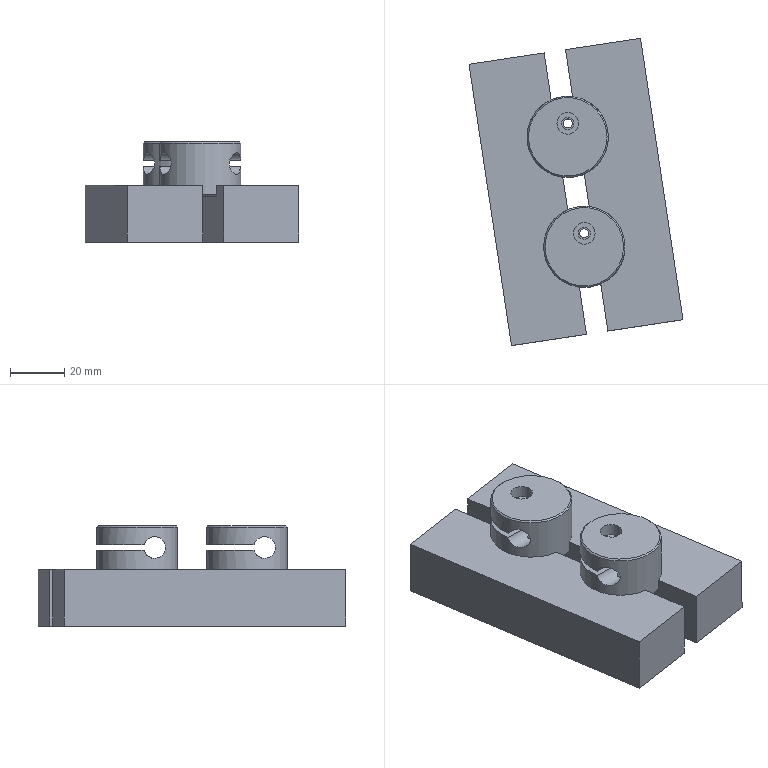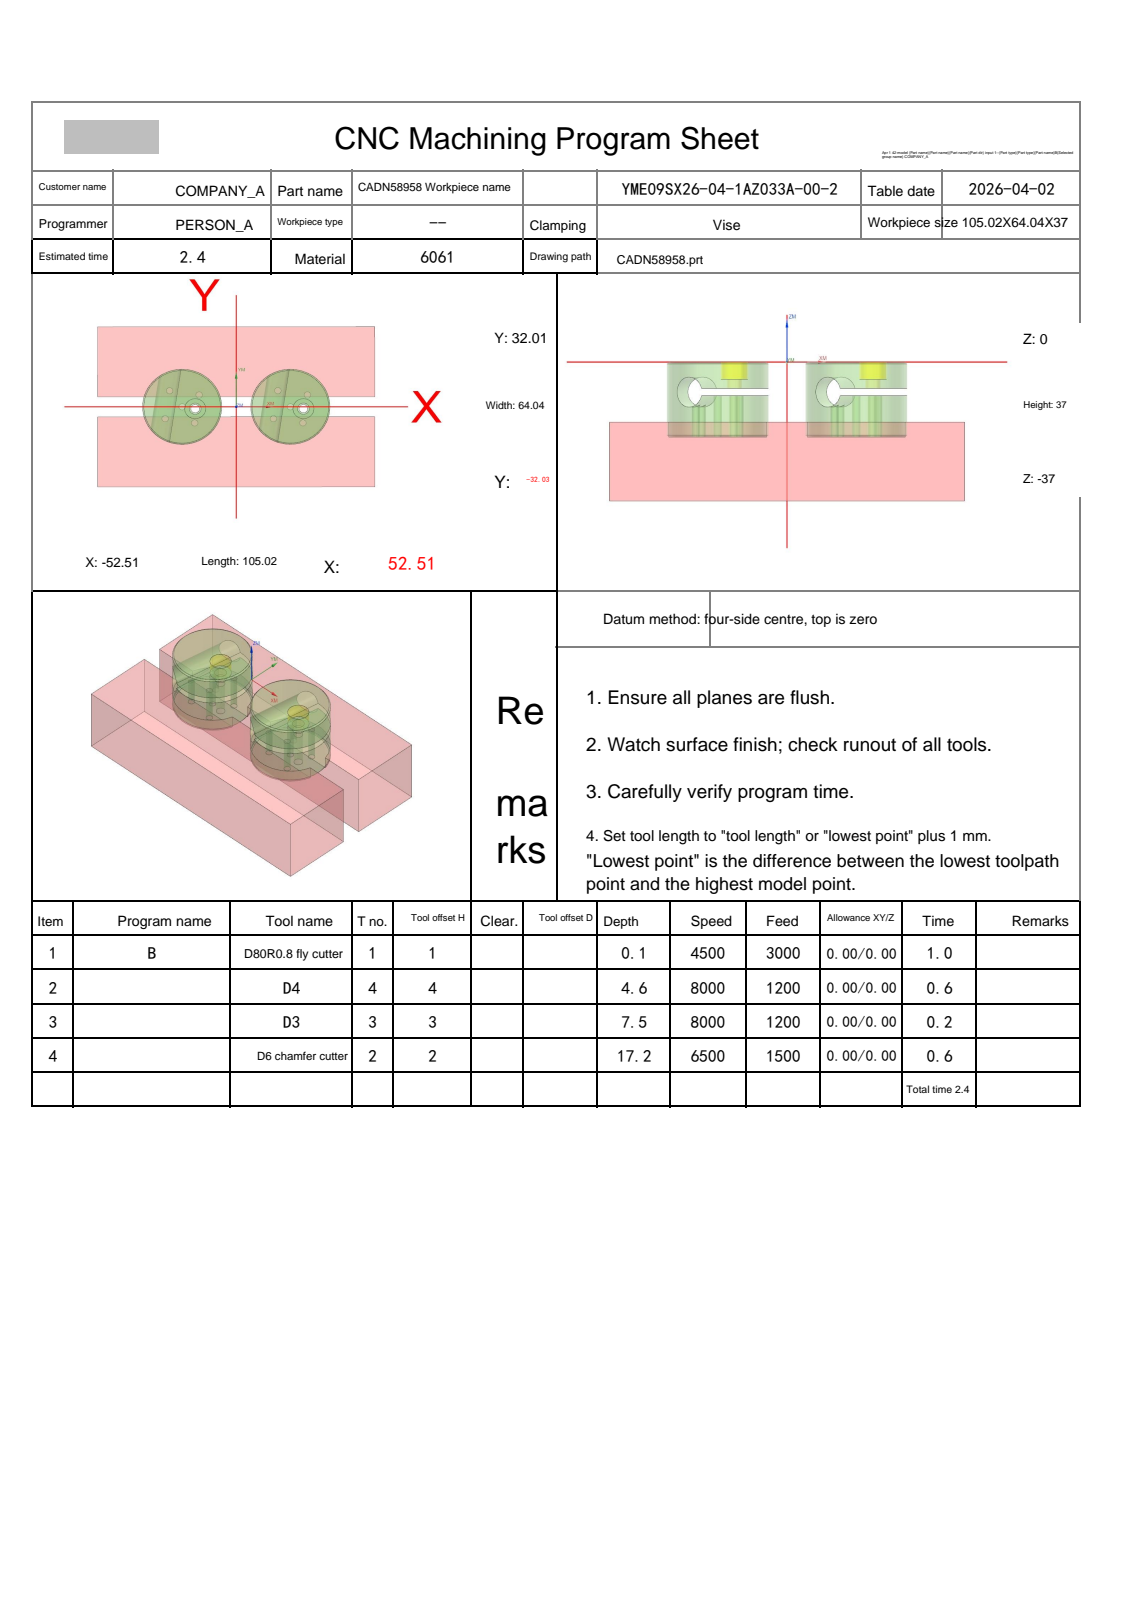NC program | NX | posted by the shop | part box 78.946 x 113.372 x 37 mm
Whole program:
%
O0001
(Machine time: 3.09 MIN)
(===Total Tool:4===)
(T1=D80R0.8 fly cutter D=80.  R=0.8  D-  H01 Z=0.    )
(T4=D4      D=4.   R=0.   D4  H04 Z=-4.6  )
(T3=D3      D=3.   R=0.   D3  H03 Z=-7.5  )
(T2=D6 chamfer cutter   D=6.   R=0.   D-  H02 Z=-17.2 )
G80 G90 G17 G49 G40
G91 G28 Z0
M01
N1 T01 M06
(D80R0.8 fly cutter  D=80. R=0.8 H=01 ce=0.20 di=0.10)
G00 G90 G54 X-104.523 Y-.009 M03 S4500
G43 H01 Z50.
M08
Z6.011
G01 Z4.011 F3000.
X-92.523
X92.529
X104.529
Z6.011
G00 Z7.5
X-104.523
Z5.522
G01 Z3.522
X-92.523
X92.529
X104.529
Z5.522
G00 Z7.011
X-104.523
Z5.033
G01 Z3.033
X-92.523
X92.529
X104.529
Z5.033
G00 Z6.522
X-104.523
Z4.544
G01 Z2.544
X-92.523
X92.529
X104.529
Z4.544
G00 Z6.033
X-104.523
Z4.056
G01 Z2.056
X-92.523
X92.529
X104.529
Z4.056
G00 Z5.544
X-104.523
Z3.567
G01 Z1.567
X-92.523
X92.529
X104.529
Z3.567
G00 Z5.056
X-104.523
Z3.078
G01 Z1.078
X-92.523
X92.529
X104.529
Z3.078
G00 Z4.567
X-104.523
Z2.589
G01 Z.589
X-92.523
X92.529
X104.529
Z2.589
G00 Z4.078
X-104.523
Z2.1
G01 Z.1
X-92.523
X92.529
X104.529
Z2.1
G00 Z50.
G00 G90 X-104.523 Y-.009 M03 S4500
Z50.
Z2.
G01 Z0.0 F1000.
X-92.523
X92.529
X104.529
Z2.
G00 Z50.
G91 G28 Z0.0
M05
M09
G91 G28 Z0.0
M01
N2 T04 M06
(D4  D=4. R=0. H=04 ce=0.05 di=0.00)
G00 G90 G54 X25.447 Y-.745 M03 S8000
G43 H04 Z50.
M08
Z.5
G01 X25.302 Y-.734 F1200.
G03 X24.327 Y-1.709 I0.0 J-.975
X25.157 Y-2.673 I.975 J0.0
X25.157 Y-2.673 Z.2 I.29 J1.928
X25.157 Y-2.673 Z-.1 I.29 J1.928
X25.157 Y-2.673 Z-.4 I.29 J1.928
X25.157 Y-2.673 Z-.7 I.29 J1.928
X25.157 Y-2.673 Z-1. I.29 J1.928
X25.157 Y-2.673 Z-1.3 I.29 J1.928
X25.157 Y-2.673 Z-1.6 I.29 J1.928
X25.157 Y-2.673 Z-1.9 I.29 J1.928
X25.157 Y-2.673 Z-2.2 I.29 J1.928
X25.157 Y-2.673 Z-2.5 I.29 J1.928
X25.157 Y-2.673 Z-2.8 I.29 J1.928
X25.157 Y-2.673 Z-3.1 I.29 J1.928
X25.157 Y-2.673 Z-3.4 I.29 J1.928
X25.157 Y-2.673 Z-3.7 I.29 J1.928
X25.157 Y-2.673 Z-4. I.29 J1.928
X25.157 Y-2.673 Z-4.3 I.29 J1.928
X25.157 Y-2.673 Z-4.6 I.29 J1.928
X25.447 Y-2.695 I.29 J1.928
X27.397 Y-.745 I0.0 J1.95
X25.447 Y1.205 I-1.95 J0.0
X23.497 Y-.745 I0.0 J-1.95
X25.157 Y-2.673 I1.95 J0.0
G01 X25.302 Y-2.684
G03 X26.277 Y-1.709 I0.0 J.975
X25.447 Y-.745 I-.975 J0.0
G00 Z50.
X-15.553 Y-.76
Z.5
G01 X-15.698 Y-.749
G03 X-16.673 Y-1.724 I0.0 J-.975
X-15.843 Y-2.688 I.975 J0.0
X-15.843 Y-2.688 Z.2 I.29 J1.928
X-15.843 Y-2.688 Z-.1 I.29 J1.928
X-15.843 Y-2.688 Z-.4 I.29 J1.928
X-15.843 Y-2.688 Z-.7 I.29 J1.928
X-15.843 Y-2.688 Z-1. I.29 J1.928
X-15.843 Y-2.688 Z-1.3 I.29 J1.928
X-15.843 Y-2.688 Z-1.6 I.29 J1.928
X-15.843 Y-2.688 Z-1.9 I.29 J1.928
X-15.843 Y-2.688 Z-2.2 I.29 J1.928
X-15.843 Y-2.688 Z-2.5 I.29 J1.928
X-15.843 Y-2.688 Z-2.8 I.29 J1.928
X-15.843 Y-2.688 Z-3.1 I.29 J1.928
X-15.843 Y-2.688 Z-3.4 I.29 J1.928
X-15.843 Y-2.688 Z-3.7 I.29 J1.928
X-15.843 Y-2.688 Z-4. I.29 J1.928
X-15.843 Y-2.688 Z-4.3 I.29 J1.928
X-15.843 Y-2.688 Z-4.6 I.29 J1.928
X-15.553 Y-2.71 I.29 J1.928
X-13.603 Y-.76 I0.0 J1.95
X-15.553 Y1.19 I-1.95 J0.0
X-17.503 Y-.76 I0.0 J-1.95
X-15.843 Y-2.688 I1.95 J0.0
G01 X-15.698 Y-2.699
G03 X-14.723 Y-1.724 I0.0 J.975
X-15.553 Y-.76 I-.975 J0.0
G00 Z50.
G00 G90 X25.447 Y-.745 M03 S8000
Z50.
Z.5
G41 D04
G01 X25.247 Y-.755 F500.
G03 X24.307 Y-1.744 I.049 J-.989
X25.15 Y-2.723 I.99 J0.0
X25.15 Y-2.723 Z-4.5 I.298 J1.978
X25.4 Y-2.745 Z-4.6 I.298 J1.978
G01 X25.447
G03 X27.447 Y-.745 I0.0 J2.
X25.447 Y1.255 I-2. J0.0
X23.447 Y-.745 I0.0 J-2.
X25.4 Y-2.745 I2. J0.0
G01 X25.423
G03 X26.413 Y-1.755 I0.0 J.99
X25.642 Y-.789 I-.99 J0.0
G01 G40 X25.447 Y-.745
G00 Z50.
X-15.553 Y-.76
Z.5
G41 D04
G01 X-15.753 Y-.77
G03 X-16.693 Y-1.759 I.049 J-.989
X-15.85 Y-2.738 I.99 J0.0
X-15.85 Y-2.738 Z-4.5 I.298 J1.978
X-15.6 Y-2.76 Z-4.6 I.298 J1.978
G01 X-15.553
G03 X-13.553 Y-.76 I0.0 J2.
X-15.553 Y1.24 I-2. J0.0
X-17.553 Y-.76 I0.0 J-2.
X-15.6 Y-2.76 I2. J0.0
G01 X-15.577
G03 X-14.587 Y-1.77 I0.0 J.99
X-15.358 Y-.804 I-.99 J0.0
G01 G40 X-15.553 Y-.76
G00 Z50.
G91 G28 Z0.0
M05
M09
G91 G28 Z0.0
M01
N3 T03 M06
(D3  D=3. R=0. H=03 ce=0.05 di=0.00)
G00 G90 G54 X25.447 Y-.745 M03 S8000
G43 H03 Z50.
M08
Z-4.1
G01 X25.395 Y-.741 F1200.
G03 X25.045 Y-1.091 I0.0 J-.35
X25.343 Y-1.437 I.35 J0.0
X25.343 Y-1.437 Z-4.4 I.104 J.692
X25.343 Y-1.437 Z-4.7 I.104 J.692
X25.343 Y-1.437 Z-5. I.104 J.692
X25.343 Y-1.437 Z-5.3 I.104 J.692
X25.343 Y-1.437 Z-5.6 I.104 J.692
X25.343 Y-1.437 Z-5.9 I.104 J.692
X25.343 Y-1.437 Z-6.2 I.104 J.692
X25.343 Y-1.437 Z-6.5 I.104 J.692
X25.343 Y-1.437 Z-6.8 I.104 J.692
X25.343 Y-1.437 Z-7.1 I.104 J.692
X25.343 Y-1.437 Z-7.4 I.104 J.692
X26.099 Y-.489 Z-7.5 I.104 J.692
X25.447 Y-.045 I-.652 J-.256
X24.747 Y-.745 I0.0 J-.7
X25.447 Y-1.445 I.7 J0.0
X26.147 Y-.745 I0.0 J.7
X26.099 Y-.489 I-.7 J0.0
X25.773 Y-.267 I-.326 J-.128
X25.423 Y-.617 I0.0 J-.35
G01 X25.447 Y-.745
G00 Z50.
X-15.553 Y-.76
Z-4.1
G01 X-15.605 Y-.756
G03 X-15.955 Y-1.106 I0.0 J-.35
X-15.657 Y-1.452 I.35 J0.0
X-15.657 Y-1.452 Z-4.4 I.104 J.692
X-15.657 Y-1.452 Z-4.7 I.104 J.692
X-15.657 Y-1.452 Z-5. I.104 J.692
X-15.657 Y-1.452 Z-5.3 I.104 J.692
X-15.657 Y-1.452 Z-5.6 I.104 J.692
X-15.657 Y-1.452 Z-5.9 I.104 J.692
X-15.657 Y-1.452 Z-6.2 I.104 J.692
X-15.657 Y-1.452 Z-6.5 I.104 J.692
X-15.657 Y-1.452 Z-6.8 I.104 J.692
X-15.657 Y-1.452 Z-7.1 I.104 J.692
X-15.657 Y-1.452 Z-7.4 I.104 J.692
X-14.901 Y-.504 Z-7.5 I.104 J.692
X-15.553 Y-.06 I-.652 J-.256
X-16.253 Y-.76 I0.0 J-.7
X-15.553 Y-1.46 I.7 J0.0
X-14.853 Y-.76 I0.0 J.7
X-14.901 Y-.504 I-.7 J0.0
X-15.227 Y-.282 I-.326 J-.128
X-15.577 Y-.632 I0.0 J-.35
G01 X-15.553 Y-.76
G00 Z50.
G00 G90 X25.447 Y-.745 M03 S8000
Z50.
Z-4.1
G41 D03
G01 X25.261 Y-.818 F500.
G03 X25.039 Y-1.142 I.127 J-.325
X25.336 Y-1.487 I.348 J0.0
X24.824 Y-.328 Z-7.5 I.112 J.742
X24.697 Y-.745 I.624 J-.417
X25.447 Y-1.495 I.75 J0.0
X26.197 Y-.745 I0.0 J.75
X25.447 Y.005 I-.75 J0.0
X24.824 Y-.328 I0.0 J-.75
X24.765 Y-.522 I.29 J-.194
X25.113 Y-.87 I.348 J0.0
G01 X25.268 Y-.834
G40 X25.447 Y-.745
G00 Z50.
X-15.553 Y-.76
Z-4.1
G41 D03
G01 X-15.739 Y-.833
G03 X-15.961 Y-1.157 I.127 J-.325
X-15.664 Y-1.502 I.348 J0.0
X-16.176 Y-.343 Z-7.5 I.112 J.742
X-16.303 Y-.76 I.624 J-.417
X-15.553 Y-1.51 I.75 J0.0
X-14.803 Y-.76 I0.0 J.75
X-15.553 Y-.01 I-.75 J0.0
X-16.176 Y-.343 I0.0 J-.75
X-16.235 Y-.537 I.29 J-.194
X-15.887 Y-.885 I.348 J0.0
G01 X-15.732 Y-.849
G40 X-15.553 Y-.76
G00 Z50.
G91 G28 Z0.0
M05
M09
G91 G28 Z0.0
M01
N4 T02 M06
(D6 chamfer cutter  D=6. R=0. H=02 ce=0.00 di=0.00)
G00 G90 G54 X26.261 Y1.967 M03 S6500
G43 H02 Z50.
M08
Z.24
G01 Z-1.2 F1500.
G03 X25.991 Y2.187 I-1.396 J-1.432
G01 X25.948 Y2.22
X25.894 Y2.221
G03 X25.447 Y2.255 I-.446 J-2.967
X22.447 Y-.745 I0.0 J-3.
X25.447 Y-3.745 I3. J0.0
X28.447 Y-.745 I0.0 J3.
X25.894 Y2.221 I-3. J0.0
G01 X25.841 Y2.236
X25.79 Y2.218
G03 X25.467 Y2.086 I.59 J-1.911
G01 Z.24
G00 Z10.
X-14.739 Y1.952
Z.24
G01 Z-1.2
G03 X-15.009 Y2.172 I-1.396 J-1.432
G01 X-15.052 Y2.205
X-15.106 Y2.206
G03 X-15.553 Y2.24 I-.446 J-2.967
X-18.553 Y-.76 I0.0 J-3.
X-15.553 Y-3.76 I3. J0.0
X-12.553 Y-.76 I0.0 J3.
X-15.106 Y2.206 I-3. J0.0
G01 X-15.159 Y2.221
X-15.21 Y2.203
G03 X-15.533 Y2.071 I.59 J-1.911
G01 Z.24
G00 Z10.
X-2.528 Y-2.964
Z-2.127
G01 Z-17.2
X-2.471 Y-3.004
X-2.451 Y-3.01
X2.459 Y-3.008
X2.479 Y-3.002
X2.536 Y-2.962
Z-2.127
G00 Z10.
X38.447 Y-2.949
Z-2.127
G01 Z-17.2
X38.504 Y-2.989
X38.524 Y-2.995
X52.504 Y-2.989
G02 X53.504 Y-3.989 I0.0 J-1.
G01 X53.515 Y-31.989
G02 X52.515 Y-32.989 I-1. J0.0
G01 X.015 Y-33.009
X-52.485 Y-33.028
G02 X-53.485 Y-32.028 I0.0 J1.
G01 X-53.496 Y-4.028
G02 X-52.496 Y-3.028 I1. J0.0
G01 X-38.516 Y-3.023
X-38.496 Y-3.017
X-38.439 Y-2.977
Z-2.127
G00 Z10.
X2.534 Y2.947
Z-2.127
G01 Z-17.2
X2.477 Y2.987
X2.457 Y2.992
X-2.453 Y2.99
X-2.473 Y2.985
X-2.53 Y2.945
Z-2.127
G00 Z10.
X-38.476 Y2.932
Z-2.127
G01 Z-17.2
X-38.533 Y2.972
X-38.553 Y2.977
X-52.498 Y2.972
G02 X-53.499 Y3.972 I0.0 J1.
G01 X-53.509 Y31.972
G02 X-52.509 Y32.972 I1. J0.0
G01 X-.009 Y32.991
X52.491 Y33.011
G02 X53.491 Y32.011 I0.0 J-1.
G01 X53.501 Y4.011
G02 X52.502 Y3.011 I-1. J0.0
G01 X38.522 Y3.005
X38.512 Y3.003
X38.484 Y2.983
Z-2.127
G00 Z50.
G00 G90 X-21.82 Y-16.864 M03 S6500
Z50.
Z.3
G01 Z-1.2 F1500.
X-21.812 Y-16.728
G03 X-22.833 Y-15.541 I-1.2 J0.0
G02 X-36.197 Y-.016 I2.336 J15.525
X-20.497 Y15.684 I15.7 J0.0
X-4.797 Y-.016 I0.0 J-15.7
X-14.532 Y-14.539 I-15.7 J0.0
X-16.342 Y-15.156 I-5.965 J14.523
G01 X-16.444 Y-15.184
X-16.499 Y-15.199
X-16.612 Y-15.228
X-16.624 Y-15.231
G02 X-20.497 Y-15.716 I-3.873 J15.215
X-22.833 Y-15.541 I0.0 J15.7
X-23.228 Y-15.477 I2.336 J15.525
G03 X-23.437 Y-15.459 I-.209 J-1.182
X-24.61 Y-16.408 I0.0 J-1.2
G01 Z.3
G00 Z50.
G00 G90 X21.825 Y16.847 M03 S6500
Z50.
Z.3
G01 Z-1.2 F1500.
X21.818 Y16.711
G03 X22.839 Y15.524 I1.2 J0.0
G02 X36.203 Y-.001 I-2.336 J-15.525
X29.128 Y-13.12 I-15.7 J0.0
G01 X29.03 Y-13.184
G02 X20.503 Y-15.701 I-8.527 J13.183
X4.803 Y-.001 I0.0 J15.7
X20.503 Y15.699 I15.7 J0.0
X22.839 Y15.524 I0.0 J-15.7
X23.234 Y15.459 I-2.336 J-15.525
G03 X23.442 Y15.441 I.209 J1.182
X24.616 Y16.391 I0.0 J1.2
G01 Z.3
G00 Z50.
M05
M09
G91 G28 Z0.0
G91 G28 Y0.0
M30
%